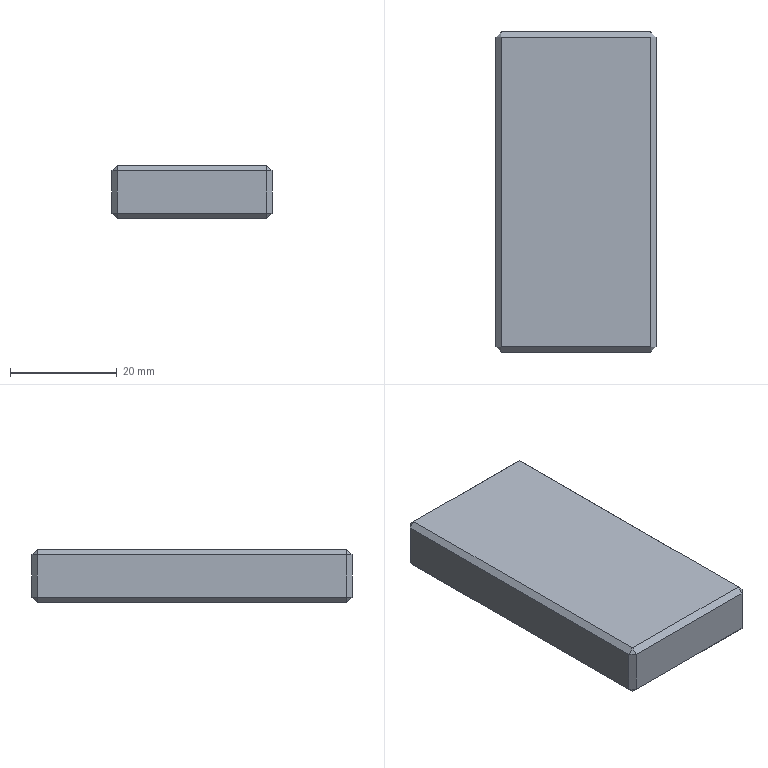Part | STEP file | Planar support spacer block | 1 solid | 26 faces | box 30 x 60 x 10 mm | volume 17805 mm3 | plane 26
STEP:
#1=CARTESIAN_POINT('',(0.,0.,0.));
#2=DIRECTION('',(0.,0.,1.));
#3=DIRECTION('',(1.,0.,0.));
#4=AXIS2_PLACEMENT_3D('',#1,#2,#3);
#5=CARTESIAN_POINT('',(15.,29.,9.));
#6=VERTEX_POINT('',#5);
#7=CARTESIAN_POINT('',(15.,-29.,9.));
#8=VERTEX_POINT('',#7);
#9=CARTESIAN_POINT('',(15.,-30.,9.));
#10=DIRECTION('',(0.,-1.,0.));
#11=VECTOR('',#10,1.);
#12=LINE('',#9,#11);
#13=CARTESIAN_POINT('',(15.,30.,10.));
#14=DIRECTION('',(-1.,0.,0.));
#15=DIRECTION('',(0.,-1.,0.));
#16=AXIS2_PLACEMENT_3D('',#13,#14,#15);
#17=PLANE('',#16);
#18=CARTESIAN_POINT('',(60.,-1.));
#19=DIRECTION('',(1.,0.));
#20=VECTOR('',#19,1.);
#21=LINE('',#18,#20);
#22=(GEOMETRIC_REPRESENTATION_CONTEXT(2)PARAMETRIC_REPRESENTATION_CONTEXT()REPRESENTATION_CONTEXT('',''));
#23=DEFINITIONAL_REPRESENTATION('',(#21),#22);
#24=PCURVE('',#17,#23);
#25=CARTESIAN_POINT('',(14.,0.,10.));
#26=DIRECTION('',(0.7071,0.,0.7071));
#27=DIRECTION('',(0.,-1.,0.));
#28=AXIS2_PLACEMENT_3D('',#25,#26,#27);
#29=PLANE('',#28);
#30=CARTESIAN_POINT('',(30.,1.414));
#31=DIRECTION('',(1.,0.));
#32=VECTOR('',#31,1.);
#33=LINE('',#30,#32);
#34=(GEOMETRIC_REPRESENTATION_CONTEXT(2)PARAMETRIC_REPRESENTATION_CONTEXT()REPRESENTATION_CONTEXT('',''));
#35=DEFINITIONAL_REPRESENTATION('',(#33),#34);
#36=PCURVE('',#29,#35);
#37=SURFACE_CURVE('',#12,(#24,#36),.PCURVE_S1.);
#38=EDGE_CURVE('',#6,#8,#37,.T.);
#39=ORIENTED_EDGE('',*,*,#38,.T.);
#40=CARTESIAN_POINT('',(15.,-29.,1.));
#41=VERTEX_POINT('',#40);
#42=CARTESIAN_POINT('',(15.,-29.,10.));
#43=DIRECTION('',(0.,0.,-1.));
#44=VECTOR('',#43,1.);
#45=LINE('',#42,#44);
#46=CARTESIAN_POINT('',(59.,0.));
#47=DIRECTION('',(0.,-1.));
#48=VECTOR('',#47,1.);
#49=LINE('',#46,#48);
#50=(GEOMETRIC_REPRESENTATION_CONTEXT(2)PARAMETRIC_REPRESENTATION_CONTEXT()REPRESENTATION_CONTEXT('',''));
#51=DEFINITIONAL_REPRESENTATION('',(#49),#50);
#52=PCURVE('',#17,#51);
#53=CARTESIAN_POINT('',(15.,-29.,10.));
#54=DIRECTION('',(-0.7071,0.7071,0.));
#55=DIRECTION('',(0.,0.,-1.));
#56=AXIS2_PLACEMENT_3D('',#53,#54,#55);
#57=PLANE('',#56);
#58=CARTESIAN_POINT('',(0.,0.));
#59=DIRECTION('',(1.,0.));
#60=VECTOR('',#59,1.);
#61=LINE('',#58,#60);
#62=(GEOMETRIC_REPRESENTATION_CONTEXT(2)PARAMETRIC_REPRESENTATION_CONTEXT()REPRESENTATION_CONTEXT('',''));
#63=DEFINITIONAL_REPRESENTATION('',(#61),#62);
#64=PCURVE('',#57,#63);
#65=SURFACE_CURVE('',#45,(#52,#64),.PCURVE_S1.);
#66=EDGE_CURVE('',#8,#41,#65,.T.);
#67=ORIENTED_EDGE('',*,*,#66,.T.);
#68=CARTESIAN_POINT('',(15.,29.,1.));
#69=VERTEX_POINT('',#68);
#70=CARTESIAN_POINT('',(15.,30.,1.));
#71=DIRECTION('',(0.,1.,0.));
#72=VECTOR('',#71,1.);
#73=LINE('',#70,#72);
#74=CARTESIAN_POINT('',(0.,-9.));
#75=DIRECTION('',(-1.,0.));
#76=VECTOR('',#75,1.);
#77=LINE('',#74,#76);
#78=(GEOMETRIC_REPRESENTATION_CONTEXT(2)PARAMETRIC_REPRESENTATION_CONTEXT()REPRESENTATION_CONTEXT('',''));
#79=DEFINITIONAL_REPRESENTATION('',(#77),#78);
#80=PCURVE('',#17,#79);
#81=CARTESIAN_POINT('',(15.,30.,1.));
#82=DIRECTION('',(-0.7071,0.,0.7071));
#83=DIRECTION('',(0.,1.,0.));
#84=AXIS2_PLACEMENT_3D('',#81,#82,#83);
#85=PLANE('',#84);
#86=CARTESIAN_POINT('',(0.,0.));
#87=DIRECTION('',(1.,0.));
#88=VECTOR('',#87,1.);
#89=LINE('',#86,#88);
#90=(GEOMETRIC_REPRESENTATION_CONTEXT(2)PARAMETRIC_REPRESENTATION_CONTEXT()REPRESENTATION_CONTEXT('',''));
#91=DEFINITIONAL_REPRESENTATION('',(#89),#90);
#92=PCURVE('',#85,#91);
#93=SURFACE_CURVE('',#73,(#80,#92),.PCURVE_S1.);
#94=EDGE_CURVE('',#41,#69,#93,.T.);
#95=ORIENTED_EDGE('',*,*,#94,.T.);
#96=CARTESIAN_POINT('',(15.,29.,10.));
#97=DIRECTION('',(0.,0.,1.));
#98=VECTOR('',#97,1.);
#99=LINE('',#96,#98);
#100=CARTESIAN_POINT('',(1.,0.));
#101=DIRECTION('',(0.,1.));
#102=VECTOR('',#101,1.);
#103=LINE('',#100,#102);
#104=(GEOMETRIC_REPRESENTATION_CONTEXT(2)PARAMETRIC_REPRESENTATION_CONTEXT()REPRESENTATION_CONTEXT('',''));
#105=DEFINITIONAL_REPRESENTATION('',(#103),#104);
#106=PCURVE('',#17,#105);
#107=CARTESIAN_POINT('',(14.,30.,10.));
#108=DIRECTION('',(-0.7071,-0.7071,0.));
#109=DIRECTION('',(0.,0.,-1.));
#110=AXIS2_PLACEMENT_3D('',#107,#108,#109);
#111=PLANE('',#110);
#112=CARTESIAN_POINT('',(0.,1.414));
#113=DIRECTION('',(-1.,0.));
#114=VECTOR('',#113,1.);
#115=LINE('',#112,#114);
#116=(GEOMETRIC_REPRESENTATION_CONTEXT(2)PARAMETRIC_REPRESENTATION_CONTEXT()REPRESENTATION_CONTEXT('',''));
#117=DEFINITIONAL_REPRESENTATION('',(#115),#116);
#118=PCURVE('',#111,#117);
#119=SURFACE_CURVE('',#99,(#106,#118),.PCURVE_S1.);
#120=EDGE_CURVE('',#69,#6,#119,.T.);
#121=ORIENTED_EDGE('',*,*,#120,.T.);
#122=EDGE_LOOP('',(#39,#67,#95,#121));
#123=FACE_BOUND('',#122,.T.);
#124=ADVANCED_FACE('',(#123),#17,.F.);
#125=CARTESIAN_POINT('',(14.,30.,9.));
#126=VERTEX_POINT('',#125);
#127=CARTESIAN_POINT('',(14.,30.,1.));
#128=VERTEX_POINT('',#127);
#129=CARTESIAN_POINT('',(14.,30.,10.));
#130=DIRECTION('',(0.,0.,-1.));
#131=VECTOR('',#130,1.);
#132=LINE('',#129,#131);
#133=CARTESIAN_POINT('',(-15.,30.,10.));
#134=DIRECTION('',(0.,-1.,0.));
#135=DIRECTION('',(0.,0.,-1.));
#136=AXIS2_PLACEMENT_3D('',#133,#134,#135);
#137=PLANE('',#136);
#138=CARTESIAN_POINT('',(0.,29.));
#139=DIRECTION('',(1.,0.));
#140=VECTOR('',#139,1.);
#141=LINE('',#138,#140);
#142=(GEOMETRIC_REPRESENTATION_CONTEXT(2)PARAMETRIC_REPRESENTATION_CONTEXT()REPRESENTATION_CONTEXT('',''));
#143=DEFINITIONAL_REPRESENTATION('',(#141),#142);
#144=PCURVE('',#137,#143);
#145=CARTESIAN_POINT('',(0.,0.));
#146=DIRECTION('',(1.,0.));
#147=VECTOR('',#146,1.);
#148=LINE('',#145,#147);
#149=(GEOMETRIC_REPRESENTATION_CONTEXT(2)PARAMETRIC_REPRESENTATION_CONTEXT()REPRESENTATION_CONTEXT('',''));
#150=DEFINITIONAL_REPRESENTATION('',(#148),#149);
#151=PCURVE('',#111,#150);
#152=SURFACE_CURVE('',#132,(#144,#151),.PCURVE_S1.);
#153=EDGE_CURVE('',#126,#128,#152,.T.);
#154=ORIENTED_EDGE('',*,*,#153,.T.);
#155=CARTESIAN_POINT('',(-14.,30.,1.));
#156=VERTEX_POINT('',#155);
#157=CARTESIAN_POINT('',(-15.,30.,1.));
#158=DIRECTION('',(-1.,0.,0.));
#159=VECTOR('',#158,1.);
#160=LINE('',#157,#159);
#161=CARTESIAN_POINT('',(9.,0.));
#162=DIRECTION('',(0.,-1.));
#163=VECTOR('',#162,1.);
#164=LINE('',#161,#163);
#165=(GEOMETRIC_REPRESENTATION_CONTEXT(2)PARAMETRIC_REPRESENTATION_CONTEXT()REPRESENTATION_CONTEXT('',''));
#166=DEFINITIONAL_REPRESENTATION('',(#164),#165);
#167=PCURVE('',#137,#166);
#168=CARTESIAN_POINT('',(-15.,30.,1.));
#169=DIRECTION('',(0.,-0.7071,0.7071));
#170=DIRECTION('',(-1.,0.,0.));
#171=AXIS2_PLACEMENT_3D('',#168,#169,#170);
#172=PLANE('',#171);
#173=CARTESIAN_POINT('',(0.,0.));
#174=DIRECTION('',(1.,0.));
#175=VECTOR('',#174,1.);
#176=LINE('',#173,#175);
#177=(GEOMETRIC_REPRESENTATION_CONTEXT(2)PARAMETRIC_REPRESENTATION_CONTEXT()REPRESENTATION_CONTEXT('',''));
#178=DEFINITIONAL_REPRESENTATION('',(#176),#177);
#179=PCURVE('',#172,#178);
#180=SURFACE_CURVE('',#160,(#167,#179),.PCURVE_S1.);
#181=EDGE_CURVE('',#128,#156,#180,.T.);
#182=ORIENTED_EDGE('',*,*,#181,.T.);
#183=CARTESIAN_POINT('',(-14.,30.,9.));
#184=VERTEX_POINT('',#183);
#185=CARTESIAN_POINT('',(-14.,30.,10.));
#186=DIRECTION('',(0.,0.,1.));
#187=VECTOR('',#186,1.);
#188=LINE('',#185,#187);
#189=CARTESIAN_POINT('',(0.,1.));
#190=DIRECTION('',(-1.,0.));
#191=VECTOR('',#190,1.);
#192=LINE('',#189,#191);
#193=(GEOMETRIC_REPRESENTATION_CONTEXT(2)PARAMETRIC_REPRESENTATION_CONTEXT()REPRESENTATION_CONTEXT('',''));
#194=DEFINITIONAL_REPRESENTATION('',(#192),#193);
#195=PCURVE('',#137,#194);
#196=CARTESIAN_POINT('',(-15.,29.,10.));
#197=DIRECTION('',(0.7071,-0.7071,0.));
#198=DIRECTION('',(0.,0.,-1.));
#199=AXIS2_PLACEMENT_3D('',#196,#197,#198);
#200=PLANE('',#199);
#201=CARTESIAN_POINT('',(0.,1.414));
#202=DIRECTION('',(-1.,0.));
#203=VECTOR('',#202,1.);
#204=LINE('',#201,#203);
#205=(GEOMETRIC_REPRESENTATION_CONTEXT(2)PARAMETRIC_REPRESENTATION_CONTEXT()REPRESENTATION_CONTEXT('',''));
#206=DEFINITIONAL_REPRESENTATION('',(#204),#205);
#207=PCURVE('',#200,#206);
#208=SURFACE_CURVE('',#188,(#195,#207),.PCURVE_S1.);
#209=EDGE_CURVE('',#156,#184,#208,.T.);
#210=ORIENTED_EDGE('',*,*,#209,.T.);
#211=CARTESIAN_POINT('',(15.,30.,9.));
#212=DIRECTION('',(1.,0.,0.));
#213=VECTOR('',#212,1.);
#214=LINE('',#211,#213);
#215=CARTESIAN_POINT('',(1.,30.));
#216=DIRECTION('',(0.,1.));
#217=VECTOR('',#216,1.);
#218=LINE('',#215,#217);
#219=(GEOMETRIC_REPRESENTATION_CONTEXT(2)PARAMETRIC_REPRESENTATION_CONTEXT()REPRESENTATION_CONTEXT('',''));
#220=DEFINITIONAL_REPRESENTATION('',(#218),#219);
#221=PCURVE('',#137,#220);
#222=CARTESIAN_POINT('',(0.,29.,10.));
#223=DIRECTION('',(0.,0.7071,0.7071));
#224=DIRECTION('',(1.,0.,0.));
#225=AXIS2_PLACEMENT_3D('',#222,#223,#224);
#226=PLANE('',#225);
#227=CARTESIAN_POINT('',(15.,1.414));
#228=DIRECTION('',(1.,0.));
#229=VECTOR('',#228,1.);
#230=LINE('',#227,#229);
#231=(GEOMETRIC_REPRESENTATION_CONTEXT(2)PARAMETRIC_REPRESENTATION_CONTEXT()REPRESENTATION_CONTEXT('',''));
#232=DEFINITIONAL_REPRESENTATION('',(#230),#231);
#233=PCURVE('',#226,#232);
#234=SURFACE_CURVE('',#214,(#221,#233),.PCURVE_S1.);
#235=EDGE_CURVE('',#184,#126,#234,.T.);
#236=ORIENTED_EDGE('',*,*,#235,.T.);
#237=EDGE_LOOP('',(#154,#182,#210,#236));
#238=FACE_BOUND('',#237,.T.);
#239=ADVANCED_FACE('',(#238),#137,.F.);
#240=CARTESIAN_POINT('',(-15.,29.,9.));
#241=VERTEX_POINT('',#240);
#242=CARTESIAN_POINT('',(-15.,29.,1.));
#243=VERTEX_POINT('',#242);
#244=CARTESIAN_POINT('',(-15.,29.,10.));
#245=DIRECTION('',(0.,0.,-1.));
#246=VECTOR('',#245,1.);
#247=LINE('',#244,#246);
#248=CARTESIAN_POINT('',(-15.,30.,10.));
#249=DIRECTION('',(1.,0.,0.));
#250=DIRECTION('',(0.,1.,0.));
#251=AXIS2_PLACEMENT_3D('',#248,#249,#250);
#252=PLANE('',#251);
#253=CARTESIAN_POINT('',(-1.,0.));
#254=DIRECTION('',(0.,-1.));
#255=VECTOR('',#254,1.);
#256=LINE('',#253,#255);
#257=(GEOMETRIC_REPRESENTATION_CONTEXT(2)PARAMETRIC_REPRESENTATION_CONTEXT()REPRESENTATION_CONTEXT('',''));
#258=DEFINITIONAL_REPRESENTATION('',(#256),#257);
#259=PCURVE('',#252,#258);
#260=CARTESIAN_POINT('',(0.,0.));
#261=DIRECTION('',(1.,0.));
#262=VECTOR('',#261,1.);
#263=LINE('',#260,#262);
#264=(GEOMETRIC_REPRESENTATION_CONTEXT(2)PARAMETRIC_REPRESENTATION_CONTEXT()REPRESENTATION_CONTEXT('',''));
#265=DEFINITIONAL_REPRESENTATION('',(#263),#264);
#266=PCURVE('',#200,#265);
#267=SURFACE_CURVE('',#247,(#259,#266),.PCURVE_S1.);
#268=EDGE_CURVE('',#241,#243,#267,.T.);
#269=ORIENTED_EDGE('',*,*,#268,.T.);
#270=CARTESIAN_POINT('',(-15.,-29.,1.));
#271=VERTEX_POINT('',#270);
#272=CARTESIAN_POINT('',(-15.,30.,1.));
#273=DIRECTION('',(0.,-1.,0.));
#274=VECTOR('',#273,1.);
#275=LINE('',#272,#274);
#276=CARTESIAN_POINT('',(0.,-9.));
#277=DIRECTION('',(-1.,0.));
#278=VECTOR('',#277,1.);
#279=LINE('',#276,#278);
#280=(GEOMETRIC_REPRESENTATION_CONTEXT(2)PARAMETRIC_REPRESENTATION_CONTEXT()REPRESENTATION_CONTEXT('',''));
#281=DEFINITIONAL_REPRESENTATION('',(#279),#280);
#282=PCURVE('',#252,#281);
#283=CARTESIAN_POINT('',(-15.,30.,1.));
#284=DIRECTION('',(0.7071,0.,0.7071));
#285=DIRECTION('',(0.,-1.,0.));
#286=AXIS2_PLACEMENT_3D('',#283,#284,#285);
#287=PLANE('',#286);
#288=CARTESIAN_POINT('',(0.,0.));
#289=DIRECTION('',(1.,0.));
#290=VECTOR('',#289,1.);
#291=LINE('',#288,#290);
#292=(GEOMETRIC_REPRESENTATION_CONTEXT(2)PARAMETRIC_REPRESENTATION_CONTEXT()REPRESENTATION_CONTEXT('',''));
#293=DEFINITIONAL_REPRESENTATION('',(#291),#292);
#294=PCURVE('',#287,#293);
#295=SURFACE_CURVE('',#275,(#282,#294),.PCURVE_S1.);
#296=EDGE_CURVE('',#243,#271,#295,.T.);
#297=ORIENTED_EDGE('',*,*,#296,.T.);
#298=CARTESIAN_POINT('',(-15.,-29.,9.));
#299=VERTEX_POINT('',#298);
#300=CARTESIAN_POINT('',(-15.,-29.,10.));
#301=DIRECTION('',(0.,0.,1.));
#302=VECTOR('',#301,1.);
#303=LINE('',#300,#302);
#304=CARTESIAN_POINT('',(-59.,0.));
#305=DIRECTION('',(0.,1.));
#306=VECTOR('',#305,1.);
#307=LINE('',#304,#306);
#308=(GEOMETRIC_REPRESENTATION_CONTEXT(2)PARAMETRIC_REPRESENTATION_CONTEXT()REPRESENTATION_CONTEXT('',''));
#309=DEFINITIONAL_REPRESENTATION('',(#307),#308);
#310=PCURVE('',#252,#309);
#311=CARTESIAN_POINT('',(-14.,-30.,10.));
#312=DIRECTION('',(0.7071,0.7071,0.));
#313=DIRECTION('',(0.,0.,-1.));
#314=AXIS2_PLACEMENT_3D('',#311,#312,#313);
#315=PLANE('',#314);
#316=CARTESIAN_POINT('',(0.,1.414));
#317=DIRECTION('',(-1.,0.));
#318=VECTOR('',#317,1.);
#319=LINE('',#316,#318);
#320=(GEOMETRIC_REPRESENTATION_CONTEXT(2)PARAMETRIC_REPRESENTATION_CONTEXT()REPRESENTATION_CONTEXT('',''));
#321=DEFINITIONAL_REPRESENTATION('',(#319),#320);
#322=PCURVE('',#315,#321);
#323=SURFACE_CURVE('',#303,(#310,#322),.PCURVE_S1.);
#324=EDGE_CURVE('',#271,#299,#323,.T.);
#325=ORIENTED_EDGE('',*,*,#324,.T.);
#326=CARTESIAN_POINT('',(-15.,30.,9.));
#327=DIRECTION('',(0.,1.,0.));
#328=VECTOR('',#327,1.);
#329=LINE('',#326,#328);
#330=CARTESIAN_POINT('',(0.,-1.));
#331=DIRECTION('',(1.,0.));
#332=VECTOR('',#331,1.);
#333=LINE('',#330,#332);
#334=(GEOMETRIC_REPRESENTATION_CONTEXT(2)PARAMETRIC_REPRESENTATION_CONTEXT()REPRESENTATION_CONTEXT('',''));
#335=DEFINITIONAL_REPRESENTATION('',(#333),#334);
#336=PCURVE('',#252,#335);
#337=CARTESIAN_POINT('',(-14.,0.,10.));
#338=DIRECTION('',(-0.7071,0.,0.7071));
#339=DIRECTION('',(0.,1.,0.));
#340=AXIS2_PLACEMENT_3D('',#337,#338,#339);
#341=PLANE('',#340);
#342=CARTESIAN_POINT('',(30.,1.414));
#343=DIRECTION('',(1.,0.));
#344=VECTOR('',#343,1.);
#345=LINE('',#342,#344);
#346=(GEOMETRIC_REPRESENTATION_CONTEXT(2)PARAMETRIC_REPRESENTATION_CONTEXT()REPRESENTATION_CONTEXT('',''));
#347=DEFINITIONAL_REPRESENTATION('',(#345),#346);
#348=PCURVE('',#341,#347);
#349=SURFACE_CURVE('',#329,(#336,#348),.PCURVE_S1.);
#350=EDGE_CURVE('',#299,#241,#349,.T.);
#351=ORIENTED_EDGE('',*,*,#350,.T.);
#352=EDGE_LOOP('',(#269,#297,#325,#351));
#353=FACE_BOUND('',#352,.T.);
#354=ADVANCED_FACE('',(#353),#252,.F.);
#355=CARTESIAN_POINT('',(-14.,-30.,9.));
#356=VERTEX_POINT('',#355);
#357=CARTESIAN_POINT('',(-14.,-30.,1.));
#358=VERTEX_POINT('',#357);
#359=CARTESIAN_POINT('',(-14.,-30.,10.));
#360=DIRECTION('',(0.,0.,-1.));
#361=VECTOR('',#360,1.);
#362=LINE('',#359,#361);
#363=CARTESIAN_POINT('',(-15.,-30.,10.));
#364=DIRECTION('',(0.,1.,0.));
#365=DIRECTION('',(0.,0.,1.));
#366=AXIS2_PLACEMENT_3D('',#363,#364,#365);
#367=PLANE('',#366);
#368=CARTESIAN_POINT('',(0.,1.));
#369=DIRECTION('',(-1.,0.));
#370=VECTOR('',#369,1.);
#371=LINE('',#368,#370);
#372=(GEOMETRIC_REPRESENTATION_CONTEXT(2)PARAMETRIC_REPRESENTATION_CONTEXT()REPRESENTATION_CONTEXT('',''));
#373=DEFINITIONAL_REPRESENTATION('',(#371),#372);
#374=PCURVE('',#367,#373);
#375=CARTESIAN_POINT('',(0.,0.));
#376=DIRECTION('',(1.,0.));
#377=VECTOR('',#376,1.);
#378=LINE('',#375,#377);
#379=(GEOMETRIC_REPRESENTATION_CONTEXT(2)PARAMETRIC_REPRESENTATION_CONTEXT()REPRESENTATION_CONTEXT('',''));
#380=DEFINITIONAL_REPRESENTATION('',(#378),#379);
#381=PCURVE('',#315,#380);
#382=SURFACE_CURVE('',#362,(#374,#381),.PCURVE_S1.);
#383=EDGE_CURVE('',#356,#358,#382,.T.);
#384=ORIENTED_EDGE('',*,*,#383,.T.);
#385=CARTESIAN_POINT('',(14.,-30.,1.));
#386=VERTEX_POINT('',#385);
#387=CARTESIAN_POINT('',(-15.,-30.,1.));
#388=DIRECTION('',(1.,0.,0.));
#389=VECTOR('',#388,1.);
#390=LINE('',#387,#389);
#391=CARTESIAN_POINT('',(-9.,0.));
#392=DIRECTION('',(0.,1.));
#393=VECTOR('',#392,1.);
#394=LINE('',#391,#393);
#395=(GEOMETRIC_REPRESENTATION_CONTEXT(2)PARAMETRIC_REPRESENTATION_CONTEXT()REPRESENTATION_CONTEXT('',''));
#396=DEFINITIONAL_REPRESENTATION('',(#394),#395);
#397=PCURVE('',#367,#396);
#398=CARTESIAN_POINT('',(-15.,-30.,1.));
#399=DIRECTION('',(0.,0.7071,0.7071));
#400=DIRECTION('',(1.,0.,0.));
#401=AXIS2_PLACEMENT_3D('',#398,#399,#400);
#402=PLANE('',#401);
#403=CARTESIAN_POINT('',(0.,0.));
#404=DIRECTION('',(1.,0.));
#405=VECTOR('',#404,1.);
#406=LINE('',#403,#405);
#407=(GEOMETRIC_REPRESENTATION_CONTEXT(2)PARAMETRIC_REPRESENTATION_CONTEXT()REPRESENTATION_CONTEXT('',''));
#408=DEFINITIONAL_REPRESENTATION('',(#406),#407);
#409=PCURVE('',#402,#408);
#410=SURFACE_CURVE('',#390,(#397,#409),.PCURVE_S1.);
#411=EDGE_CURVE('',#358,#386,#410,.T.);
#412=ORIENTED_EDGE('',*,*,#411,.T.);
#413=CARTESIAN_POINT('',(14.,-30.,9.));
#414=VERTEX_POINT('',#413);
#415=CARTESIAN_POINT('',(14.,-30.,10.));
#416=DIRECTION('',(0.,0.,1.));
#417=VECTOR('',#416,1.);
#418=LINE('',#415,#417);
#419=CARTESIAN_POINT('',(0.,29.));
#420=DIRECTION('',(1.,0.));
#421=VECTOR('',#420,1.);
#422=LINE('',#419,#421);
#423=(GEOMETRIC_REPRESENTATION_CONTEXT(2)PARAMETRIC_REPRESENTATION_CONTEXT()REPRESENTATION_CONTEXT('',''));
#424=DEFINITIONAL_REPRESENTATION('',(#422),#423);
#425=PCURVE('',#367,#424);
#426=CARTESIAN_POINT('',(0.,1.414));
#427=DIRECTION('',(-1.,0.));
#428=VECTOR('',#427,1.);
#429=LINE('',#426,#428);
#430=(GEOMETRIC_REPRESENTATION_CONTEXT(2)PARAMETRIC_REPRESENTATION_CONTEXT()REPRESENTATION_CONTEXT('',''));
#431=DEFINITIONAL_REPRESENTATION('',(#429),#430);
#432=PCURVE('',#57,#431);
#433=SURFACE_CURVE('',#418,(#425,#432),.PCURVE_S1.);
#434=EDGE_CURVE('',#386,#414,#433,.T.);
#435=ORIENTED_EDGE('',*,*,#434,.T.);
#436=CARTESIAN_POINT('',(-15.,-30.,9.));
#437=DIRECTION('',(-1.,0.,0.));
#438=VECTOR('',#437,1.);
#439=LINE('',#436,#438);
#440=CARTESIAN_POINT('',(-1.,0.));
#441=DIRECTION('',(0.,-1.));
#442=VECTOR('',#441,1.);
#443=LINE('',#440,#442);
#444=(GEOMETRIC_REPRESENTATION_CONTEXT(2)PARAMETRIC_REPRESENTATION_CONTEXT()REPRESENTATION_CONTEXT('',''));
#445=DEFINITIONAL_REPRESENTATION('',(#443),#444);
#446=PCURVE('',#367,#445);
#447=CARTESIAN_POINT('',(0.,-29.,10.));
#448=DIRECTION('',(0.,-0.7071,0.7071));
#449=DIRECTION('',(-1.,0.,0.));
#450=AXIS2_PLACEMENT_3D('',#447,#448,#449);
#451=PLANE('',#450);
#452=CARTESIAN_POINT('',(15.,1.414));
#453=DIRECTION('',(1.,0.));
#454=VECTOR('',#453,1.);
#455=LINE('',#452,#454);
#456=(GEOMETRIC_REPRESENTATION_CONTEXT(2)PARAMETRIC_REPRESENTATION_CONTEXT()REPRESENTATION_CONTEXT('',''));
#457=DEFINITIONAL_REPRESENTATION('',(#455),#456);
#458=PCURVE('',#451,#457);
#459=SURFACE_CURVE('',#439,(#446,#458),.PCURVE_S1.);
#460=EDGE_CURVE('',#414,#356,#459,.T.);
#461=ORIENTED_EDGE('',*,*,#460,.T.);
#462=EDGE_LOOP('',(#384,#412,#435,#461));
#463=FACE_BOUND('',#462,.T.);
#464=ADVANCED_FACE('',(#463),#367,.F.);
#465=CARTESIAN_POINT('',(-14.,-29.,10.));
#466=VERTEX_POINT('',#465);
#467=CARTESIAN_POINT('',(14.,-29.,10.));
#468=VERTEX_POINT('',#467);
#469=CARTESIAN_POINT('',(15.,-29.,10.));
#470=DIRECTION('',(1.,0.,0.));
#471=VECTOR('',#470,1.);
#472=LINE('',#469,#471);
#473=CARTESIAN_POINT('',(0.,0.,10.));
#474=DIRECTION('',(0.,0.,1.));
#475=DIRECTION('',(1.,0.,0.));
#476=AXIS2_PLACEMENT_3D('',#473,#474,#475);
#477=PLANE('',#476);
#478=CARTESIAN_POINT('',(15.,-29.));
#479=DIRECTION('',(1.,0.));
#480=VECTOR('',#479,1.);
#481=LINE('',#478,#480);
#482=(GEOMETRIC_REPRESENTATION_CONTEXT(2)PARAMETRIC_REPRESENTATION_CONTEXT()REPRESENTATION_CONTEXT('',''));
#483=DEFINITIONAL_REPRESENTATION('',(#481),#482);
#484=PCURVE('',#477,#483);
#485=CARTESIAN_POINT('',(-15.,0.));
#486=DIRECTION('',(-1.,0.));
#487=VECTOR('',#486,1.);
#488=LINE('',#485,#487);
#489=(GEOMETRIC_REPRESENTATION_CONTEXT(2)PARAMETRIC_REPRESENTATION_CONTEXT()REPRESENTATION_CONTEXT('',''));
#490=DEFINITIONAL_REPRESENTATION('',(#488),#489);
#491=PCURVE('',#451,#490);
#492=SURFACE_CURVE('',#472,(#484,#491),.PCURVE_S1.);
#493=EDGE_CURVE('',#466,#468,#492,.T.);
#494=ORIENTED_EDGE('',*,*,#493,.T.);
#495=CARTESIAN_POINT('',(14.,29.,10.));
#496=VERTEX_POINT('',#495);
#497=CARTESIAN_POINT('',(14.,30.,10.));
#498=DIRECTION('',(0.,1.,0.));
#499=VECTOR('',#498,1.);
#500=LINE('',#497,#499);
#501=CARTESIAN_POINT('',(14.,30.));
#502=DIRECTION('',(0.,1.));
#503=VECTOR('',#502,1.);
#504=LINE('',#501,#503);
#505=(GEOMETRIC_REPRESENTATION_CONTEXT(2)PARAMETRIC_REPRESENTATION_CONTEXT()REPRESENTATION_CONTEXT('',''));
#506=DEFINITIONAL_REPRESENTATION('',(#504),#505);
#507=PCURVE('',#477,#506);
#508=CARTESIAN_POINT('',(-30.,0.));
#509=DIRECTION('',(-1.,0.));
#510=VECTOR('',#509,1.);
#511=LINE('',#508,#510);
#512=(GEOMETRIC_REPRESENTATION_CONTEXT(2)PARAMETRIC_REPRESENTATION_CONTEXT()REPRESENTATION_CONTEXT('',''));
#513=DEFINITIONAL_REPRESENTATION('',(#511),#512);
#514=PCURVE('',#29,#513);
#515=SURFACE_CURVE('',#500,(#507,#514),.PCURVE_S1.);
#516=EDGE_CURVE('',#468,#496,#515,.T.);
#517=ORIENTED_EDGE('',*,*,#516,.T.);
#518=CARTESIAN_POINT('',(-14.,29.,10.));
#519=VERTEX_POINT('',#518);
#520=CARTESIAN_POINT('',(-15.,29.,10.));
#521=DIRECTION('',(-1.,0.,0.));
#522=VECTOR('',#521,1.);
#523=LINE('',#520,#522);
#524=CARTESIAN_POINT('',(-15.,29.));
#525=DIRECTION('',(-1.,0.));
#526=VECTOR('',#525,1.);
#527=LINE('',#524,#526);
#528=(GEOMETRIC_REPRESENTATION_CONTEXT(2)PARAMETRIC_REPRESENTATION_CONTEXT()REPRESENTATION_CONTEXT('',''));
#529=DEFINITIONAL_REPRESENTATION('',(#527),#528);
#530=PCURVE('',#477,#529);
#531=CARTESIAN_POINT('',(-15.,0.));
#532=DIRECTION('',(-1.,0.));
#533=VECTOR('',#532,1.);
#534=LINE('',#531,#533);
#535=(GEOMETRIC_REPRESENTATION_CONTEXT(2)PARAMETRIC_REPRESENTATION_CONTEXT()REPRESENTATION_CONTEXT('',''));
#536=DEFINITIONAL_REPRESENTATION('',(#534),#535);
#537=PCURVE('',#226,#536);
#538=SURFACE_CURVE('',#523,(#530,#537),.PCURVE_S1.);
#539=EDGE_CURVE('',#496,#519,#538,.T.);
#540=ORIENTED_EDGE('',*,*,#539,.T.);
#541=CARTESIAN_POINT('',(-14.,-30.,10.));
#542=DIRECTION('',(0.,-1.,0.));
#543=VECTOR('',#542,1.);
#544=LINE('',#541,#543);
#545=CARTESIAN_POINT('',(-14.,-30.));
#546=DIRECTION('',(0.,-1.));
#547=VECTOR('',#546,1.);
#548=LINE('',#545,#547);
#549=(GEOMETRIC_REPRESENTATION_CONTEXT(2)PARAMETRIC_REPRESENTATION_CONTEXT()REPRESENTATION_CONTEXT('',''));
#550=DEFINITIONAL_REPRESENTATION('',(#548),#549);
#551=PCURVE('',#477,#550);
#552=CARTESIAN_POINT('',(-30.,0.));
#553=DIRECTION('',(-1.,0.));
#554=VECTOR('',#553,1.);
#555=LINE('',#552,#554);
#556=(GEOMETRIC_REPRESENTATION_CONTEXT(2)PARAMETRIC_REPRESENTATION_CONTEXT()REPRESENTATION_CONTEXT('',''));
#557=DEFINITIONAL_REPRESENTATION('',(#555),#556);
#558=PCURVE('',#341,#557);
#559=SURFACE_CURVE('',#544,(#551,#558),.PCURVE_S1.);
#560=EDGE_CURVE('',#519,#466,#559,.T.);
#561=ORIENTED_EDGE('',*,*,#560,.T.);
#562=EDGE_LOOP('',(#494,#517,#540,#561));
#563=FACE_BOUND('',#562,.T.);
#564=ADVANCED_FACE('',(#563),#477,.T.);
#565=CARTESIAN_POINT('',(-14.,29.,0.));
#566=VERTEX_POINT('',#565);
#567=CARTESIAN_POINT('',(14.,29.,0.));
#568=VERTEX_POINT('',#567);
#569=CARTESIAN_POINT('',(0.,29.,0.));
#570=DIRECTION('',(1.,0.,0.));
#571=VECTOR('',#570,1.);
#572=LINE('',#569,#571);
#573=CARTESIAN_POINT('',(0.,0.,0.));
#574=DIRECTION('',(0.,0.,1.));
#575=DIRECTION('',(1.,0.,0.));
#576=AXIS2_PLACEMENT_3D('',#573,#574,#575);
#577=PLANE('',#576);
#578=CARTESIAN_POINT('',(0.,29.));
#579=DIRECTION('',(1.,0.));
#580=VECTOR('',#579,1.);
#581=LINE('',#578,#580);
#582=(GEOMETRIC_REPRESENTATION_CONTEXT(2)PARAMETRIC_REPRESENTATION_CONTEXT()REPRESENTATION_CONTEXT('',''));
#583=DEFINITIONAL_REPRESENTATION('',(#581),#582);
#584=PCURVE('',#577,#583);
#585=CARTESIAN_POINT('',(-15.,1.414));
#586=DIRECTION('',(-1.,0.));
#587=VECTOR('',#586,1.);
#588=LINE('',#585,#587);
#589=(GEOMETRIC_REPRESENTATION_CONTEXT(2)PARAMETRIC_REPRESENTATION_CONTEXT()REPRESENTATION_CONTEXT('',''));
#590=DEFINITIONAL_REPRESENTATION('',(#588),#589);
#591=PCURVE('',#172,#590);
#592=SURFACE_CURVE('',#572,(#584,#591),.PCURVE_S1.);
#593=EDGE_CURVE('',#566,#568,#592,.T.);
#594=ORIENTED_EDGE('',*,*,#593,.T.);
#595=CARTESIAN_POINT('',(14.,-29.,0.));
#596=VERTEX_POINT('',#595);
#597=CARTESIAN_POINT('',(14.,0.,0.));
#598=DIRECTION('',(0.,-1.,0.));
#599=VECTOR('',#598,1.);
#600=LINE('',#597,#599);
#601=CARTESIAN_POINT('',(14.,0.));
#602=DIRECTION('',(0.,-1.));
#603=VECTOR('',#602,1.);
#604=LINE('',#601,#603);
#605=(GEOMETRIC_REPRESENTATION_CONTEXT(2)PARAMETRIC_REPRESENTATION_CONTEXT()REPRESENTATION_CONTEXT('',''));
#606=DEFINITIONAL_REPRESENTATION('',(#604),#605);
#607=PCURVE('',#577,#606);
#608=CARTESIAN_POINT('',(-30.,1.414));
#609=DIRECTION('',(-1.,0.));
#610=VECTOR('',#609,1.);
#611=LINE('',#608,#610);
#612=(GEOMETRIC_REPRESENTATION_CONTEXT(2)PARAMETRIC_REPRESENTATION_CONTEXT()REPRESENTATION_CONTEXT('',''));
#613=DEFINITIONAL_REPRESENTATION('',(#611),#612);
#614=PCURVE('',#85,#613);
#615=SURFACE_CURVE('',#600,(#607,#614),.PCURVE_S1.);
#616=EDGE_CURVE('',#568,#596,#615,.T.);
#617=ORIENTED_EDGE('',*,*,#616,.T.);
#618=CARTESIAN_POINT('',(-14.,-29.,0.));
#619=VERTEX_POINT('',#618);
#620=CARTESIAN_POINT('',(0.,-29.,0.));
#621=DIRECTION('',(-1.,0.,0.));
#622=VECTOR('',#621,1.);
#623=LINE('',#620,#622);
#624=CARTESIAN_POINT('',(0.,-29.));
#625=DIRECTION('',(-1.,0.));
#626=VECTOR('',#625,1.);
#627=LINE('',#624,#626);
#628=(GEOMETRIC_REPRESENTATION_CONTEXT(2)PARAMETRIC_REPRESENTATION_CONTEXT()REPRESENTATION_CONTEXT('',''));
#629=DEFINITIONAL_REPRESENTATION('',(#627),#628);
#630=PCURVE('',#577,#629);
#631=CARTESIAN_POINT('',(15.,1.414));
#632=DIRECTION('',(-1.,0.));
#633=VECTOR('',#632,1.);
#634=LINE('',#631,#633);
#635=(GEOMETRIC_REPRESENTATION_CONTEXT(2)PARAMETRIC_REPRESENTATION_CONTEXT()REPRESENTATION_CONTEXT('',''));
#636=DEFINITIONAL_REPRESENTATION('',(#634),#635);
#637=PCURVE('',#402,#636);
#638=SURFACE_CURVE('',#623,(#630,#637),.PCURVE_S1.);
#639=EDGE_CURVE('',#596,#619,#638,.T.);
#640=ORIENTED_EDGE('',*,*,#639,.T.);
#641=CARTESIAN_POINT('',(-14.,0.,0.));
#642=DIRECTION('',(0.,1.,0.));
#643=VECTOR('',#642,1.);
#644=LINE('',#641,#643);
#645=CARTESIAN_POINT('',(-14.,0.));
#646=DIRECTION('',(0.,1.));
#647=VECTOR('',#646,1.);
#648=LINE('',#645,#647);
#649=(GEOMETRIC_REPRESENTATION_CONTEXT(2)PARAMETRIC_REPRESENTATION_CONTEXT()REPRESENTATION_CONTEXT('',''));
#650=DEFINITIONAL_REPRESENTATION('',(#648),#649);
#651=PCURVE('',#577,#650);
#652=CARTESIAN_POINT('',(30.,1.414));
#653=DIRECTION('',(-1.,0.));
#654=VECTOR('',#653,1.);
#655=LINE('',#652,#654);
#656=(GEOMETRIC_REPRESENTATION_CONTEXT(2)PARAMETRIC_REPRESENTATION_CONTEXT()REPRESENTATION_CONTEXT('',''));
#657=DEFINITIONAL_REPRESENTATION('',(#655),#656);
#658=PCURVE('',#287,#657);
#659=SURFACE_CURVE('',#644,(#651,#658),.PCURVE_S1.);
#660=EDGE_CURVE('',#619,#566,#659,.T.);
#661=ORIENTED_EDGE('',*,*,#660,.T.);
#662=EDGE_LOOP('',(#594,#617,#640,#661));
#663=FACE_BOUND('',#662,.T.);
#664=ADVANCED_FACE('',(#663),#577,.F.);
#665=CARTESIAN_POINT('',(-14.5,-29.,9.5));
#666=DIRECTION('',(-0.7071,0.,-0.7071));
#667=VECTOR('',#666,1.);
#668=LINE('',#665,#667);
#669=CARTESIAN_POINT('',(-29.,0.7071));
#670=DIRECTION('',(0.,1.));
#671=VECTOR('',#670,1.);
#672=LINE('',#669,#671);
#673=(GEOMETRIC_REPRESENTATION_CONTEXT(2)PARAMETRIC_REPRESENTATION_CONTEXT()REPRESENTATION_CONTEXT('',''));
#674=DEFINITIONAL_REPRESENTATION('',(#672),#673);
#675=PCURVE('',#341,#674);
#676=CARTESIAN_POINT('',(-14.,-30.,9.));
#677=DIRECTION('',(-0.5774,-0.5774,0.5774));
#678=DIRECTION('',(0.7071,0.,0.7071));
#679=AXIS2_PLACEMENT_3D('',#676,#677,#678);
#680=PLANE('',#679);
#681=CARTESIAN_POINT('',(0.,1.225));
#682=DIRECTION('',(-1.,0.));
#683=VECTOR('',#682,1.);
#684=LINE('',#681,#683);
#685=(GEOMETRIC_REPRESENTATION_CONTEXT(2)PARAMETRIC_REPRESENTATION_CONTEXT()REPRESENTATION_CONTEXT('',''));
#686=DEFINITIONAL_REPRESENTATION('',(#684),#685);
#687=PCURVE('',#680,#686);
#688=SURFACE_CURVE('',#668,(#675,#687),.PCURVE_S1.);
#689=EDGE_CURVE('',#466,#299,#688,.T.);
#690=ORIENTED_EDGE('',*,*,#689,.F.);
#691=ORIENTED_EDGE('',*,*,#560,.F.);
#692=CARTESIAN_POINT('',(-15.,29.,9.));
#693=DIRECTION('',(0.7071,0.,0.7071));
#694=VECTOR('',#693,1.);
#695=LINE('',#692,#694);
#696=CARTESIAN_POINT('',(29.,1.414));
#697=DIRECTION('',(0.,-1.));
#698=VECTOR('',#697,1.);
#699=LINE('',#696,#698);
#700=(GEOMETRIC_REPRESENTATION_CONTEXT(2)PARAMETRIC_REPRESENTATION_CONTEXT()REPRESENTATION_CONTEXT('',''));
#701=DEFINITIONAL_REPRESENTATION('',(#699),#700);
#702=PCURVE('',#341,#701);
#703=CARTESIAN_POINT('',(-15.,29.,9.));
#704=DIRECTION('',(-0.5774,0.5774,0.5774));
#705=DIRECTION('',(0.7071,0.,0.7071));
#706=AXIS2_PLACEMENT_3D('',#703,#704,#705);
#707=PLANE('',#706);
#708=CARTESIAN_POINT('',(0.,0.));
#709=DIRECTION('',(1.,0.));
#710=VECTOR('',#709,1.);
#711=LINE('',#708,#710);
#712=(GEOMETRIC_REPRESENTATION_CONTEXT(2)PARAMETRIC_REPRESENTATION_CONTEXT()REPRESENTATION_CONTEXT('',''));
#713=DEFINITIONAL_REPRESENTATION('',(#711),#712);
#714=PCURVE('',#707,#713);
#715=SURFACE_CURVE('',#695,(#702,#714),.PCURVE_S1.);
#716=EDGE_CURVE('',#241,#519,#715,.T.);
#717=ORIENTED_EDGE('',*,*,#716,.F.);
#718=ORIENTED_EDGE('',*,*,#350,.F.);
#719=EDGE_LOOP('',(#690,#691,#717,#718));
#720=FACE_BOUND('',#719,.T.);
#721=ADVANCED_FACE('',(#720),#341,.T.);
#722=CARTESIAN_POINT('',(-14.,-30.,9.));
#723=DIRECTION('',(0.,-0.7071,-0.7071));
#724=VECTOR('',#723,1.);
#725=LINE('',#722,#724);
#726=CARTESIAN_POINT('',(0.,0.));
#727=DIRECTION('',(-0.5,-0.866));
#728=VECTOR('',#727,1.);
#729=LINE('',#726,#728);
#730=(GEOMETRIC_REPRESENTATION_CONTEXT(2)PARAMETRIC_REPRESENTATION_CONTEXT()REPRESENTATION_CONTEXT('',''));
#731=DEFINITIONAL_REPRESENTATION('',(#729),#730);
#732=PCURVE('',#680,#731);
#733=CARTESIAN_POINT('',(14.,1.414));
#734=DIRECTION('',(0.,1.));
#735=VECTOR('',#734,1.);
#736=LINE('',#733,#735);
#737=(GEOMETRIC_REPRESENTATION_CONTEXT(2)PARAMETRIC_REPRESENTATION_CONTEXT()REPRESENTATION_CONTEXT('',''));
#738=DEFINITIONAL_REPRESENTATION('',(#736),#737);
#739=PCURVE('',#451,#738);
#740=SURFACE_CURVE('',#725,(#732,#739),.PCURVE_S1.);
#741=EDGE_CURVE('',#466,#356,#740,.T.);
#742=ORIENTED_EDGE('',*,*,#741,.F.);
#743=ORIENTED_EDGE('',*,*,#689,.T.);
#744=CARTESIAN_POINT('',(-14.,-30.,9.));
#745=DIRECTION('',(-0.7071,0.7071,0.));
#746=VECTOR('',#745,1.);
#747=LINE('',#744,#746);
#748=CARTESIAN_POINT('',(0.,0.));
#749=DIRECTION('',(-0.5,0.866));
#750=VECTOR('',#749,1.);
#751=LINE('',#748,#750);
#752=(GEOMETRIC_REPRESENTATION_CONTEXT(2)PARAMETRIC_REPRESENTATION_CONTEXT()REPRESENTATION_CONTEXT('',''));
#753=DEFINITIONAL_REPRESENTATION('',(#751),#752);
#754=PCURVE('',#680,#753);
#755=CARTESIAN_POINT('',(1.,0.));
#756=DIRECTION('',(0.,1.));
#757=VECTOR('',#756,1.);
#758=LINE('',#755,#757);
#759=(GEOMETRIC_REPRESENTATION_CONTEXT(2)PARAMETRIC_REPRESENTATION_CONTEXT()REPRESENTATION_CONTEXT('',''));
#760=DEFINITIONAL_REPRESENTATION('',(#758),#759);
#761=PCURVE('',#315,#760);
#762=SURFACE_CURVE('',#747,(#754,#761),.PCURVE_S1.);
#763=EDGE_CURVE('',#356,#299,#762,.T.);
#764=ORIENTED_EDGE('',*,*,#763,.F.);
#765=EDGE_LOOP('',(#742,#743,#764));
#766=FACE_BOUND('',#765,.T.);
#767=ADVANCED_FACE('',(#766),#680,.T.);
#768=CARTESIAN_POINT('',(-15.,29.,9.));
#769=DIRECTION('',(0.7071,0.7071,0.));
#770=VECTOR('',#769,1.);
#771=LINE('',#768,#770);
#772=CARTESIAN_POINT('',(0.,0.));
#773=DIRECTION('',(0.5,0.866));
#774=VECTOR('',#773,1.);
#775=LINE('',#772,#774);
#776=(GEOMETRIC_REPRESENTATION_CONTEXT(2)PARAMETRIC_REPRESENTATION_CONTEXT()REPRESENTATION_CONTEXT('',''));
#777=DEFINITIONAL_REPRESENTATION('',(#775),#776);
#778=PCURVE('',#707,#777);
#779=CARTESIAN_POINT('',(1.,0.));
#780=DIRECTION('',(0.,1.));
#781=VECTOR('',#780,1.);
#782=LINE('',#779,#781);
#783=(GEOMETRIC_REPRESENTATION_CONTEXT(2)PARAMETRIC_REPRESENTATION_CONTEXT()REPRESENTATION_CONTEXT('',''));
#784=DEFINITIONAL_REPRESENTATION('',(#782),#783);
#785=PCURVE('',#200,#784);
#786=SURFACE_CURVE('',#771,(#778,#785),.PCURVE_S1.);
#787=EDGE_CURVE('',#241,#184,#786,.T.);
#788=ORIENTED_EDGE('',*,*,#787,.F.);
#789=ORIENTED_EDGE('',*,*,#716,.T.);
#790=CARTESIAN_POINT('',(-14.,29.5,9.5));
#791=DIRECTION('',(0.,-0.7071,0.7071));
#792=VECTOR('',#791,1.);
#793=LINE('',#790,#792);
#794=CARTESIAN_POINT('',(1.061,0.6124));
#795=DIRECTION('',(0.5,-0.866));
#796=VECTOR('',#795,1.);
#797=LINE('',#794,#796);
#798=(GEOMETRIC_REPRESENTATION_CONTEXT(2)PARAMETRIC_REPRESENTATION_CONTEXT()REPRESENTATION_CONTEXT('',''));
#799=DEFINITIONAL_REPRESENTATION('',(#797),#798);
#800=PCURVE('',#707,#799);
#801=CARTESIAN_POINT('',(-14.,0.7071));
#802=DIRECTION('',(0.,-1.));
#803=VECTOR('',#802,1.);
#804=LINE('',#801,#803);
#805=(GEOMETRIC_REPRESENTATION_CONTEXT(2)PARAMETRIC_REPRESENTATION_CONTEXT()REPRESENTATION_CONTEXT('',''));
#806=DEFINITIONAL_REPRESENTATION('',(#804),#805);
#807=PCURVE('',#226,#806);
#808=SURFACE_CURVE('',#793,(#800,#807),.PCURVE_S1.);
#809=EDGE_CURVE('',#184,#519,#808,.T.);
#810=ORIENTED_EDGE('',*,*,#809,.F.);
#811=EDGE_LOOP('',(#788,#789,#810));
#812=FACE_BOUND('',#811,.T.);
#813=ADVANCED_FACE('',(#812),#707,.T.);
#814=ORIENTED_EDGE('',*,*,#763,.T.);
#815=ORIENTED_EDGE('',*,*,#324,.F.);
#816=CARTESIAN_POINT('',(-15.,-29.,1.));
#817=DIRECTION('',(-0.7071,0.7071,0.));
#818=VECTOR('',#817,1.);
#819=LINE('',#816,#818);
#820=CARTESIAN_POINT('',(9.,1.414));
#821=DIRECTION('',(0.,1.));
#822=VECTOR('',#821,1.);
#823=LINE('',#820,#822);
#824=(GEOMETRIC_REPRESENTATION_CONTEXT(2)PARAMETRIC_REPRESENTATION_CONTEXT()REPRESENTATION_CONTEXT('',''));
#825=DEFINITIONAL_REPRESENTATION('',(#823),#824);
#826=PCURVE('',#315,#825);
#827=CARTESIAN_POINT('',(-15.,-29.,1.));
#828=DIRECTION('',(-0.5774,-0.5774,-0.5774));
#829=DIRECTION('',(-0.7071,0.,0.7071));
#830=AXIS2_PLACEMENT_3D('',#827,#828,#829);
#831=PLANE('',#830);
#832=CARTESIAN_POINT('',(0.,0.));
#833=DIRECTION('',(0.5,0.866));
#834=VECTOR('',#833,1.);
#835=LINE('',#832,#834);
#836=(GEOMETRIC_REPRESENTATION_CONTEXT(2)PARAMETRIC_REPRESENTATION_CONTEXT()REPRESENTATION_CONTEXT('',''));
#837=DEFINITIONAL_REPRESENTATION('',(#835),#836);
#838=PCURVE('',#831,#837);
#839=SURFACE_CURVE('',#819,(#826,#838),.PCURVE_S1.);
#840=EDGE_CURVE('',#358,#271,#839,.T.);
#841=ORIENTED_EDGE('',*,*,#840,.F.);
#842=ORIENTED_EDGE('',*,*,#383,.F.);
#843=EDGE_LOOP('',(#814,#815,#841,#842));
#844=FACE_BOUND('',#843,.T.);
#845=ADVANCED_FACE('',(#844),#315,.F.);
#846=ORIENTED_EDGE('',*,*,#741,.T.);
#847=ORIENTED_EDGE('',*,*,#460,.F.);
#848=CARTESIAN_POINT('',(14.,-29.5,9.5));
#849=DIRECTION('',(0.,-0.7071,-0.7071));
#850=VECTOR('',#849,1.);
#851=LINE('',#848,#850);
#852=CARTESIAN_POINT('',(-14.,0.7071));
#853=DIRECTION('',(0.,1.));
#854=VECTOR('',#853,1.);
#855=LINE('',#852,#854);
#856=(GEOMETRIC_REPRESENTATION_CONTEXT(2)PARAMETRIC_REPRESENTATION_CONTEXT()REPRESENTATION_CONTEXT('',''));
#857=DEFINITIONAL_REPRESENTATION('',(#855),#856);
#858=PCURVE('',#451,#857);
#859=CARTESIAN_POINT('',(15.,-29.,9.));
#860=DIRECTION('',(0.5774,-0.5774,0.5774));
#861=DIRECTION('',(0.7071,0.,-0.7071));
#862=AXIS2_PLACEMENT_3D('',#859,#860,#861);
#863=PLANE('',#862);
#864=CARTESIAN_POINT('',(-1.061,-0.6124));
#865=DIRECTION('',(0.5,-0.866));
#866=VECTOR('',#865,1.);
#867=LINE('',#864,#866);
#868=(GEOMETRIC_REPRESENTATION_CONTEXT(2)PARAMETRIC_REPRESENTATION_CONTEXT()REPRESENTATION_CONTEXT('',''));
#869=DEFINITIONAL_REPRESENTATION('',(#867),#868);
#870=PCURVE('',#863,#869);
#871=SURFACE_CURVE('',#851,(#858,#870),.PCURVE_S1.);
#872=EDGE_CURVE('',#468,#414,#871,.T.);
#873=ORIENTED_EDGE('',*,*,#872,.F.);
#874=ORIENTED_EDGE('',*,*,#493,.F.);
#875=EDGE_LOOP('',(#846,#847,#873,#874));
#876=FACE_BOUND('',#875,.T.);
#877=ADVANCED_FACE('',(#876),#451,.T.);
#878=CARTESIAN_POINT('',(14.,29.,10.));
#879=DIRECTION('',(0.7071,0.,-0.7071));
#880=VECTOR('',#879,1.);
#881=LINE('',#878,#880);
#882=CARTESIAN_POINT('',(-29.,0.));
#883=DIRECTION('',(0.,1.));
#884=VECTOR('',#883,1.);
#885=LINE('',#882,#884);
#886=(GEOMETRIC_REPRESENTATION_CONTEXT(2)PARAMETRIC_REPRESENTATION_CONTEXT()REPRESENTATION_CONTEXT('',''));
#887=DEFINITIONAL_REPRESENTATION('',(#885),#886);
#888=PCURVE('',#29,#887);
#889=CARTESIAN_POINT('',(14.,29.,10.));
#890=DIRECTION('',(0.5774,0.5774,0.5774));
#891=DIRECTION('',(0.7071,0.,-0.7071));
#892=AXIS2_PLACEMENT_3D('',#889,#890,#891);
#893=PLANE('',#892);
#894=CARTESIAN_POINT('',(0.,0.));
#895=DIRECTION('',(1.,0.));
#896=VECTOR('',#895,1.);
#897=LINE('',#894,#896);
#898=(GEOMETRIC_REPRESENTATION_CONTEXT(2)PARAMETRIC_REPRESENTATION_CONTEXT()REPRESENTATION_CONTEXT('',''));
#899=DEFINITIONAL_REPRESENTATION('',(#897),#898);
#900=PCURVE('',#893,#899);
#901=SURFACE_CURVE('',#881,(#888,#900),.PCURVE_S1.);
#902=EDGE_CURVE('',#496,#6,#901,.T.);
#903=ORIENTED_EDGE('',*,*,#902,.F.);
#904=ORIENTED_EDGE('',*,*,#516,.F.);
#905=CARTESIAN_POINT('',(15.,-29.,9.));
#906=DIRECTION('',(-0.7071,0.,0.7071));
#907=VECTOR('',#906,1.);
#908=LINE('',#905,#907);
#909=CARTESIAN_POINT('',(29.,1.414));
#910=DIRECTION('',(0.,-1.));
#911=VECTOR('',#910,1.);
#912=LINE('',#909,#911);
#913=(GEOMETRIC_REPRESENTATION_CONTEXT(2)PARAMETRIC_REPRESENTATION_CONTEXT()REPRESENTATION_CONTEXT('',''));
#914=DEFINITIONAL_REPRESENTATION('',(#912),#913);
#915=PCURVE('',#29,#914);
#916=CARTESIAN_POINT('',(0.,0.));
#917=DIRECTION('',(-1.,0.));
#918=VECTOR('',#917,1.);
#919=LINE('',#916,#918);
#920=(GEOMETRIC_REPRESENTATION_CONTEXT(2)PARAMETRIC_REPRESENTATION_CONTEXT()REPRESENTATION_CONTEXT('',''));
#921=DEFINITIONAL_REPRESENTATION('',(#919),#920);
#922=PCURVE('',#863,#921);
#923=SURFACE_CURVE('',#908,(#915,#922),.PCURVE_S1.);
#924=EDGE_CURVE('',#8,#468,#923,.T.);
#925=ORIENTED_EDGE('',*,*,#924,.F.);
#926=ORIENTED_EDGE('',*,*,#38,.F.);
#927=EDGE_LOOP('',(#903,#904,#925,#926));
#928=FACE_BOUND('',#927,.T.);
#929=ADVANCED_FACE('',(#928),#29,.T.);
#930=ORIENTED_EDGE('',*,*,#809,.T.);
#931=ORIENTED_EDGE('',*,*,#539,.F.);
#932=CARTESIAN_POINT('',(14.,29.,10.));
#933=DIRECTION('',(0.,-0.7071,0.7071));
#934=VECTOR('',#933,1.);
#935=LINE('',#932,#934);
#936=CARTESIAN_POINT('',(14.,0.));
#937=DIRECTION('',(0.,-1.));
#938=VECTOR('',#937,1.);
#939=LINE('',#936,#938);
#940=(GEOMETRIC_REPRESENTATION_CONTEXT(2)PARAMETRIC_REPRESENTATION_CONTEXT()REPRESENTATION_CONTEXT('',''));
#941=DEFINITIONAL_REPRESENTATION('',(#939),#940);
#942=PCURVE('',#226,#941);
#943=CARTESIAN_POINT('',(0.,0.));
#944=DIRECTION('',(-0.5,-0.866));
#945=VECTOR('',#944,1.);
#946=LINE('',#943,#945);
#947=(GEOMETRIC_REPRESENTATION_CONTEXT(2)PARAMETRIC_REPRESENTATION_CONTEXT()REPRESENTATION_CONTEXT('',''));
#948=DEFINITIONAL_REPRESENTATION('',(#946),#947);
#949=PCURVE('',#893,#948);
#950=SURFACE_CURVE('',#935,(#942,#949),.PCURVE_S1.);
#951=EDGE_CURVE('',#126,#496,#950,.T.);
#952=ORIENTED_EDGE('',*,*,#951,.F.);
#953=ORIENTED_EDGE('',*,*,#235,.F.);
#954=EDGE_LOOP('',(#930,#931,#952,#953));
#955=FACE_BOUND('',#954,.T.);
#956=ADVANCED_FACE('',(#955),#226,.T.);
#957=ORIENTED_EDGE('',*,*,#787,.T.);
#958=ORIENTED_EDGE('',*,*,#209,.F.);
#959=CARTESIAN_POINT('',(-14.,30.,1.));
#960=DIRECTION('',(0.7071,0.7071,0.));
#961=VECTOR('',#960,1.);
#962=LINE('',#959,#961);
#963=CARTESIAN_POINT('',(9.,1.414));
#964=DIRECTION('',(0.,1.));
#965=VECTOR('',#964,1.);
#966=LINE('',#963,#965);
#967=(GEOMETRIC_REPRESENTATION_CONTEXT(2)PARAMETRIC_REPRESENTATION_CONTEXT()REPRESENTATION_CONTEXT('',''));
#968=DEFINITIONAL_REPRESENTATION('',(#966),#967);
#969=PCURVE('',#200,#968);
#970=CARTESIAN_POINT('',(-14.,30.,1.));
#971=DIRECTION('',(-0.5774,0.5774,-0.5774));
#972=DIRECTION('',(-0.7071,0.,0.7071));
#973=AXIS2_PLACEMENT_3D('',#970,#971,#972);
#974=PLANE('',#973);
#975=CARTESIAN_POINT('',(0.,0.));
#976=DIRECTION('',(-0.5,0.866));
#977=VECTOR('',#976,1.);
#978=LINE('',#975,#977);
#979=(GEOMETRIC_REPRESENTATION_CONTEXT(2)PARAMETRIC_REPRESENTATION_CONTEXT()REPRESENTATION_CONTEXT('',''));
#980=DEFINITIONAL_REPRESENTATION('',(#978),#979);
#981=PCURVE('',#974,#980);
#982=SURFACE_CURVE('',#962,(#969,#981),.PCURVE_S1.);
#983=EDGE_CURVE('',#243,#156,#982,.T.);
#984=ORIENTED_EDGE('',*,*,#983,.F.);
#985=ORIENTED_EDGE('',*,*,#268,.F.);
#986=EDGE_LOOP('',(#957,#958,#984,#985));
#987=FACE_BOUND('',#986,.T.);
#988=ADVANCED_FACE('',(#987),#200,.F.);
#989=CARTESIAN_POINT('',(-15.,-29.,1.));
#990=DIRECTION('',(0.7071,0.,-0.7071));
#991=VECTOR('',#990,1.);
#992=LINE('',#989,#991);
#993=CARTESIAN_POINT('',(59.,0.));
#994=DIRECTION('',(0.,1.));
#995=VECTOR('',#994,1.);
#996=LINE('',#993,#995);
#997=(GEOMETRIC_REPRESENTATION_CONTEXT(2)PARAMETRIC_REPRESENTATION_CONTEXT()REPRESENTATION_CONTEXT('',''));
#998=DEFINITIONAL_REPRESENTATION('',(#996),#997);
#999=PCURVE('',#287,#998);
#1000=CARTESIAN_POINT('',(0.,0.));
#1001=DIRECTION('',(-1.,0.));
#1002=VECTOR('',#1001,1.);
#1003=LINE('',#1000,#1002);
#1004=(GEOMETRIC_REPRESENTATION_CONTEXT(2)PARAMETRIC_REPRESENTATION_CONTEXT()REPRESENTATION_CONTEXT('',''));
#1005=DEFINITIONAL_REPRESENTATION('',(#1003),#1004);
#1006=PCURVE('',#831,#1005);
#1007=SURFACE_CURVE('',#992,(#999,#1006),.PCURVE_S1.);
#1008=EDGE_CURVE('',#271,#619,#1007,.T.);
#1009=ORIENTED_EDGE('',*,*,#1008,.F.);
#1010=ORIENTED_EDGE('',*,*,#296,.F.);
#1011=CARTESIAN_POINT('',(-14.5,29.,0.5));
#1012=DIRECTION('',(-0.7071,0.,0.7071));
#1013=VECTOR('',#1012,1.);
#1014=LINE('',#1011,#1013);
#1015=CARTESIAN_POINT('',(1.,0.7071));
#1016=DIRECTION('',(0.,-1.));
#1017=VECTOR('',#1016,1.);
#1018=LINE('',#1015,#1017);
#1019=(GEOMETRIC_REPRESENTATION_CONTEXT(2)PARAMETRIC_REPRESENTATION_CONTEXT()REPRESENTATION_CONTEXT('',''));
#1020=DEFINITIONAL_REPRESENTATION('',(#1018),#1019);
#1021=PCURVE('',#287,#1020);
#1022=CARTESIAN_POINT('',(0.,-1.225));
#1023=DIRECTION('',(1.,0.));
#1024=VECTOR('',#1023,1.);
#1025=LINE('',#1022,#1024);
#1026=(GEOMETRIC_REPRESENTATION_CONTEXT(2)PARAMETRIC_REPRESENTATION_CONTEXT()REPRESENTATION_CONTEXT('',''));
#1027=DEFINITIONAL_REPRESENTATION('',(#1025),#1026);
#1028=PCURVE('',#974,#1027);
#1029=SURFACE_CURVE('',#1014,(#1021,#1028),.PCURVE_S1.);
#1030=EDGE_CURVE('',#566,#243,#1029,.T.);
#1031=ORIENTED_EDGE('',*,*,#1030,.F.);
#1032=ORIENTED_EDGE('',*,*,#660,.F.);
#1033=EDGE_LOOP('',(#1009,#1010,#1031,#1032));
#1034=FACE_BOUND('',#1033,.T.);
#1035=ADVANCED_FACE('',(#1034),#287,.F.);
#1036=ORIENTED_EDGE('',*,*,#840,.T.);
#1037=ORIENTED_EDGE('',*,*,#1008,.T.);
#1038=CARTESIAN_POINT('',(-14.,-29.5,0.5));
#1039=DIRECTION('',(0.,0.7071,-0.7071));
#1040=VECTOR('',#1039,1.);
#1041=LINE('',#1038,#1040);
#1042=CARTESIAN_POINT('',(-1.061,-0.6124));
#1043=DIRECTION('',(-0.5,0.866));
#1044=VECTOR('',#1043,1.);
#1045=LINE('',#1042,#1044);
#1046=(GEOMETRIC_REPRESENTATION_CONTEXT(2)PARAMETRIC_REPRESENTATION_CONTEXT()REPRESENTATION_CONTEXT('',''));
#1047=DEFINITIONAL_REPRESENTATION('',(#1045),#1046);
#1048=PCURVE('',#831,#1047);
#1049=CARTESIAN_POINT('',(1.,0.7071));
#1050=DIRECTION('',(0.,1.));
#1051=VECTOR('',#1050,1.);
#1052=LINE('',#1049,#1051);
#1053=(GEOMETRIC_REPRESENTATION_CONTEXT(2)PARAMETRIC_REPRESENTATION_CONTEXT()REPRESENTATION_CONTEXT('',''));
#1054=DEFINITIONAL_REPRESENTATION('',(#1052),#1053);
#1055=PCURVE('',#402,#1054);
#1056=SURFACE_CURVE('',#1041,(#1048,#1055),.PCURVE_S1.);
#1057=EDGE_CURVE('',#358,#619,#1056,.T.);
#1058=ORIENTED_EDGE('',*,*,#1057,.F.);
#1059=EDGE_LOOP('',(#1036,#1037,#1058));
#1060=FACE_BOUND('',#1059,.T.);
#1061=ADVANCED_FACE('',(#1060),#831,.T.);
#1062=ORIENTED_EDGE('',*,*,#924,.T.);
#1063=ORIENTED_EDGE('',*,*,#872,.T.);
#1064=CARTESIAN_POINT('',(15.,-29.,9.));
#1065=DIRECTION('',(-0.7071,-0.7071,0.));
#1066=VECTOR('',#1065,1.);
#1067=LINE('',#1064,#1066);
#1068=CARTESIAN_POINT('',(0.,0.));
#1069=DIRECTION('',(-0.5,-0.866));
#1070=VECTOR('',#1069,1.);
#1071=LINE('',#1068,#1070);
#1072=(GEOMETRIC_REPRESENTATION_CONTEXT(2)PARAMETRIC_REPRESENTATION_CONTEXT()REPRESENTATION_CONTEXT('',''));
#1073=DEFINITIONAL_REPRESENTATION('',(#1071),#1072);
#1074=PCURVE('',#863,#1073);
#1075=CARTESIAN_POINT('',(1.,0.));
#1076=DIRECTION('',(0.,1.));
#1077=VECTOR('',#1076,1.);
#1078=LINE('',#1075,#1077);
#1079=(GEOMETRIC_REPRESENTATION_CONTEXT(2)PARAMETRIC_REPRESENTATION_CONTEXT()REPRESENTATION_CONTEXT('',''));
#1080=DEFINITIONAL_REPRESENTATION('',(#1078),#1079);
#1081=PCURVE('',#57,#1080);
#1082=SURFACE_CURVE('',#1067,(#1074,#1081),.PCURVE_S1.);
#1083=EDGE_CURVE('',#8,#414,#1082,.T.);
#1084=ORIENTED_EDGE('',*,*,#1083,.F.);
#1085=EDGE_LOOP('',(#1062,#1063,#1084));
#1086=FACE_BOUND('',#1085,.T.);
#1087=ADVANCED_FACE('',(#1086),#863,.T.);
#1088=ORIENTED_EDGE('',*,*,#951,.T.);
#1089=ORIENTED_EDGE('',*,*,#902,.T.);
#1090=CARTESIAN_POINT('',(14.5,29.5,9.));
#1091=DIRECTION('',(0.7071,-0.7071,0.));
#1092=VECTOR('',#1091,1.);
#1093=LINE('',#1090,#1092);
#1094=CARTESIAN_POINT('',(1.061,0.6124));
#1095=DIRECTION('',(0.5,-0.866));
#1096=VECTOR('',#1095,1.);
#1097=LINE('',#1094,#1096);
#1098=(GEOMETRIC_REPRESENTATION_CONTEXT(2)PARAMETRIC_REPRESENTATION_CONTEXT()REPRESENTATION_CONTEXT('',''));
#1099=DEFINITIONAL_REPRESENTATION('',(#1097),#1098);
#1100=PCURVE('',#893,#1099);
#1101=CARTESIAN_POINT('',(1.,0.7071));
#1102=DIRECTION('',(0.,1.));
#1103=VECTOR('',#1102,1.);
#1104=LINE('',#1101,#1103);
#1105=(GEOMETRIC_REPRESENTATION_CONTEXT(2)PARAMETRIC_REPRESENTATION_CONTEXT()REPRESENTATION_CONTEXT('',''));
#1106=DEFINITIONAL_REPRESENTATION('',(#1104),#1105);
#1107=PCURVE('',#111,#1106);
#1108=SURFACE_CURVE('',#1093,(#1100,#1107),.PCURVE_S1.);
#1109=EDGE_CURVE('',#126,#6,#1108,.T.);
#1110=ORIENTED_EDGE('',*,*,#1109,.F.);
#1111=EDGE_LOOP('',(#1088,#1089,#1110));
#1112=FACE_BOUND('',#1111,.T.);
#1113=ADVANCED_FACE('',(#1112),#893,.T.);
#1114=ORIENTED_EDGE('',*,*,#1030,.T.);
#1115=ORIENTED_EDGE('',*,*,#983,.T.);
#1116=CARTESIAN_POINT('',(-14.,30.,1.));
#1117=DIRECTION('',(0.,0.7071,0.7071));
#1118=VECTOR('',#1117,1.);
#1119=LINE('',#1116,#1118);
#1120=CARTESIAN_POINT('',(0.,0.));
#1121=DIRECTION('',(0.5,0.866));
#1122=VECTOR('',#1121,1.);
#1123=LINE('',#1120,#1122);
#1124=(GEOMETRIC_REPRESENTATION_CONTEXT(2)PARAMETRIC_REPRESENTATION_CONTEXT()REPRESENTATION_CONTEXT('',''));
#1125=DEFINITIONAL_REPRESENTATION('',(#1123),#1124);
#1126=PCURVE('',#974,#1125);
#1127=CARTESIAN_POINT('',(-1.,0.));
#1128=DIRECTION('',(0.,-1.));
#1129=VECTOR('',#1128,1.);
#1130=LINE('',#1127,#1129);
#1131=(GEOMETRIC_REPRESENTATION_CONTEXT(2)PARAMETRIC_REPRESENTATION_CONTEXT()REPRESENTATION_CONTEXT('',''));
#1132=DEFINITIONAL_REPRESENTATION('',(#1130),#1131);
#1133=PCURVE('',#172,#1132);
#1134=SURFACE_CURVE('',#1119,(#1126,#1133),.PCURVE_S1.);
#1135=EDGE_CURVE('',#566,#156,#1134,.T.);
#1136=ORIENTED_EDGE('',*,*,#1135,.F.);
#1137=EDGE_LOOP('',(#1114,#1115,#1136));
#1138=FACE_BOUND('',#1137,.T.);
#1139=ADVANCED_FACE('',(#1138),#974,.T.);
#1140=ORIENTED_EDGE('',*,*,#1057,.T.);
#1141=ORIENTED_EDGE('',*,*,#639,.F.);
#1142=CARTESIAN_POINT('',(14.,-29.,0.));
#1143=DIRECTION('',(0.,0.7071,-0.7071));
#1144=VECTOR('',#1143,1.);
#1145=LINE('',#1142,#1144);
#1146=CARTESIAN_POINT('',(29.,1.414));
#1147=DIRECTION('',(0.,1.));
#1148=VECTOR('',#1147,1.);
#1149=LINE('',#1146,#1148);
#1150=(GEOMETRIC_REPRESENTATION_CONTEXT(2)PARAMETRIC_REPRESENTATION_CONTEXT()REPRESENTATION_CONTEXT('',''));
#1151=DEFINITIONAL_REPRESENTATION('',(#1149),#1150);
#1152=PCURVE('',#402,#1151);
#1153=CARTESIAN_POINT('',(14.,-29.,0.));
#1154=DIRECTION('',(0.5774,-0.5774,-0.5774));
#1155=DIRECTION('',(-0.7071,0.,-0.7071));
#1156=AXIS2_PLACEMENT_3D('',#1153,#1154,#1155);
#1157=PLANE('',#1156);
#1158=CARTESIAN_POINT('',(0.,0.));
#1159=DIRECTION('',(0.5,0.866));
#1160=VECTOR('',#1159,1.);
#1161=LINE('',#1158,#1160);
#1162=(GEOMETRIC_REPRESENTATION_CONTEXT(2)PARAMETRIC_REPRESENTATION_CONTEXT()REPRESENTATION_CONTEXT('',''));
#1163=DEFINITIONAL_REPRESENTATION('',(#1161),#1162);
#1164=PCURVE('',#1157,#1163);
#1165=SURFACE_CURVE('',#1145,(#1152,#1164),.PCURVE_S1.);
#1166=EDGE_CURVE('',#386,#596,#1165,.T.);
#1167=ORIENTED_EDGE('',*,*,#1166,.F.);
#1168=ORIENTED_EDGE('',*,*,#411,.F.);
#1169=EDGE_LOOP('',(#1140,#1141,#1167,#1168));
#1170=FACE_BOUND('',#1169,.T.);
#1171=ADVANCED_FACE('',(#1170),#402,.F.);
#1172=ORIENTED_EDGE('',*,*,#1083,.T.);
#1173=ORIENTED_EDGE('',*,*,#434,.F.);
#1174=CARTESIAN_POINT('',(14.5,-29.5,1.));
#1175=DIRECTION('',(-0.7071,-0.7071,0.));
#1176=VECTOR('',#1175,1.);
#1177=LINE('',#1174,#1176);
#1178=CARTESIAN_POINT('',(9.,0.7071));
#1179=DIRECTION('',(0.,1.));
#1180=VECTOR('',#1179,1.);
#1181=LINE('',#1178,#1180);
#1182=(GEOMETRIC_REPRESENTATION_CONTEXT(2)PARAMETRIC_REPRESENTATION_CONTEXT()REPRESENTATION_CONTEXT('',''));
#1183=DEFINITIONAL_REPRESENTATION('',(#1181),#1182);
#1184=PCURVE('',#57,#1183);
#1185=CARTESIAN_POINT('',(-1.061,-0.6124));
#1186=DIRECTION('',(0.5,-0.866));
#1187=VECTOR('',#1186,1.);
#1188=LINE('',#1185,#1187);
#1189=(GEOMETRIC_REPRESENTATION_CONTEXT(2)PARAMETRIC_REPRESENTATION_CONTEXT()REPRESENTATION_CONTEXT('',''));
#1190=DEFINITIONAL_REPRESENTATION('',(#1188),#1189);
#1191=PCURVE('',#1157,#1190);
#1192=SURFACE_CURVE('',#1177,(#1184,#1191),.PCURVE_S1.);
#1193=EDGE_CURVE('',#41,#386,#1192,.T.);
#1194=ORIENTED_EDGE('',*,*,#1193,.F.);
#1195=ORIENTED_EDGE('',*,*,#66,.F.);
#1196=EDGE_LOOP('',(#1172,#1173,#1194,#1195));
#1197=FACE_BOUND('',#1196,.T.);
#1198=ADVANCED_FACE('',(#1197),#57,.F.);
#1199=ORIENTED_EDGE('',*,*,#1109,.T.);
#1200=ORIENTED_EDGE('',*,*,#120,.F.);
#1201=CARTESIAN_POINT('',(15.,29.,1.));
#1202=DIRECTION('',(0.7071,-0.7071,0.));
#1203=VECTOR('',#1202,1.);
#1204=LINE('',#1201,#1203);
#1205=CARTESIAN_POINT('',(9.,1.414));
#1206=DIRECTION('',(0.,1.));
#1207=VECTOR('',#1206,1.);
#1208=LINE('',#1205,#1207);
#1209=(GEOMETRIC_REPRESENTATION_CONTEXT(2)PARAMETRIC_REPRESENTATION_CONTEXT()REPRESENTATION_CONTEXT('',''));
#1210=DEFINITIONAL_REPRESENTATION('',(#1208),#1209);
#1211=PCURVE('',#111,#1210);
#1212=CARTESIAN_POINT('',(15.,29.,1.));
#1213=DIRECTION('',(0.5774,0.5774,-0.5774));
#1214=DIRECTION('',(-0.7071,0.,-0.7071));
#1215=AXIS2_PLACEMENT_3D('',#1212,#1213,#1214);
#1216=PLANE('',#1215);
#1217=CARTESIAN_POINT('',(0.,0.));
#1218=DIRECTION('',(-0.5,-0.866));
#1219=VECTOR('',#1218,1.);
#1220=LINE('',#1217,#1219);
#1221=(GEOMETRIC_REPRESENTATION_CONTEXT(2)PARAMETRIC_REPRESENTATION_CONTEXT()REPRESENTATION_CONTEXT('',''));
#1222=DEFINITIONAL_REPRESENTATION('',(#1220),#1221);
#1223=PCURVE('',#1216,#1222);
#1224=SURFACE_CURVE('',#1204,(#1211,#1223),.PCURVE_S1.);
#1225=EDGE_CURVE('',#128,#69,#1224,.T.);
#1226=ORIENTED_EDGE('',*,*,#1225,.F.);
#1227=ORIENTED_EDGE('',*,*,#153,.F.);
#1228=EDGE_LOOP('',(#1199,#1200,#1226,#1227));
#1229=FACE_BOUND('',#1228,.T.);
#1230=ADVANCED_FACE('',(#1229),#111,.F.);
#1231=ORIENTED_EDGE('',*,*,#1135,.T.);
#1232=ORIENTED_EDGE('',*,*,#181,.F.);
#1233=CARTESIAN_POINT('',(14.,29.5,0.5));
#1234=DIRECTION('',(0.,0.7071,0.7071));
#1235=VECTOR('',#1234,1.);
#1236=LINE('',#1233,#1235);
#1237=CARTESIAN_POINT('',(-29.,0.7071));
#1238=DIRECTION('',(0.,-1.));
#1239=VECTOR('',#1238,1.);
#1240=LINE('',#1237,#1239);
#1241=(GEOMETRIC_REPRESENTATION_CONTEXT(2)PARAMETRIC_REPRESENTATION_CONTEXT()REPRESENTATION_CONTEXT('',''));
#1242=DEFINITIONAL_REPRESENTATION('',(#1240),#1241);
#1243=PCURVE('',#172,#1242);
#1244=CARTESIAN_POINT('',(1.061,0.6124));
#1245=DIRECTION('',(-0.5,0.866));
#1246=VECTOR('',#1245,1.);
#1247=LINE('',#1244,#1246);
#1248=(GEOMETRIC_REPRESENTATION_CONTEXT(2)PARAMETRIC_REPRESENTATION_CONTEXT()REPRESENTATION_CONTEXT('',''));
#1249=DEFINITIONAL_REPRESENTATION('',(#1247),#1248);
#1250=PCURVE('',#1216,#1249);
#1251=SURFACE_CURVE('',#1236,(#1243,#1250),.PCURVE_S1.);
#1252=EDGE_CURVE('',#568,#128,#1251,.T.);
#1253=ORIENTED_EDGE('',*,*,#1252,.F.);
#1254=ORIENTED_EDGE('',*,*,#593,.F.);
#1255=EDGE_LOOP('',(#1231,#1232,#1253,#1254));
#1256=FACE_BOUND('',#1255,.T.);
#1257=ADVANCED_FACE('',(#1256),#172,.F.);
#1258=ORIENTED_EDGE('',*,*,#1193,.T.);
#1259=ORIENTED_EDGE('',*,*,#1166,.T.);
#1260=CARTESIAN_POINT('',(14.,-29.,0.));
#1261=DIRECTION('',(-0.7071,0.,-0.7071));
#1262=VECTOR('',#1261,1.);
#1263=LINE('',#1260,#1262);
#1264=CARTESIAN_POINT('',(0.,0.));
#1265=DIRECTION('',(1.,0.));
#1266=VECTOR('',#1265,1.);
#1267=LINE('',#1264,#1266);
#1268=(GEOMETRIC_REPRESENTATION_CONTEXT(2)PARAMETRIC_REPRESENTATION_CONTEXT()REPRESENTATION_CONTEXT('',''));
#1269=DEFINITIONAL_REPRESENTATION('',(#1267),#1268);
#1270=PCURVE('',#1157,#1269);
#1271=CARTESIAN_POINT('',(-59.,1.414));
#1272=DIRECTION('',(0.,1.));
#1273=VECTOR('',#1272,1.);
#1274=LINE('',#1271,#1273);
#1275=(GEOMETRIC_REPRESENTATION_CONTEXT(2)PARAMETRIC_REPRESENTATION_CONTEXT()REPRESENTATION_CONTEXT('',''));
#1276=DEFINITIONAL_REPRESENTATION('',(#1274),#1275);
#1277=PCURVE('',#85,#1276);
#1278=SURFACE_CURVE('',#1263,(#1270,#1277),.PCURVE_S1.);
#1279=EDGE_CURVE('',#41,#596,#1278,.T.);
#1280=ORIENTED_EDGE('',*,*,#1279,.F.);
#1281=EDGE_LOOP('',(#1258,#1259,#1280));
#1282=FACE_BOUND('',#1281,.T.);
#1283=ADVANCED_FACE('',(#1282),#1157,.T.);
#1284=ORIENTED_EDGE('',*,*,#1252,.T.);
#1285=ORIENTED_EDGE('',*,*,#1225,.T.);
#1286=CARTESIAN_POINT('',(15.,29.,1.));
#1287=DIRECTION('',(0.7071,0.,0.7071));
#1288=VECTOR('',#1287,1.);
#1289=LINE('',#1286,#1288);
#1290=CARTESIAN_POINT('',(0.,0.));
#1291=DIRECTION('',(-1.,0.));
#1292=VECTOR('',#1291,1.);
#1293=LINE('',#1290,#1292);
#1294=(GEOMETRIC_REPRESENTATION_CONTEXT(2)PARAMETRIC_REPRESENTATION_CONTEXT()REPRESENTATION_CONTEXT('',''));
#1295=DEFINITIONAL_REPRESENTATION('',(#1293),#1294);
#1296=PCURVE('',#1216,#1295);
#1297=CARTESIAN_POINT('',(-1.,0.));
#1298=DIRECTION('',(0.,-1.));
#1299=VECTOR('',#1298,1.);
#1300=LINE('',#1297,#1299);
#1301=(GEOMETRIC_REPRESENTATION_CONTEXT(2)PARAMETRIC_REPRESENTATION_CONTEXT()REPRESENTATION_CONTEXT('',''));
#1302=DEFINITIONAL_REPRESENTATION('',(#1300),#1301);
#1303=PCURVE('',#85,#1302);
#1304=SURFACE_CURVE('',#1289,(#1296,#1303),.PCURVE_S1.);
#1305=EDGE_CURVE('',#568,#69,#1304,.T.);
#1306=ORIENTED_EDGE('',*,*,#1305,.F.);
#1307=EDGE_LOOP('',(#1284,#1285,#1306));
#1308=FACE_BOUND('',#1307,.T.);
#1309=ADVANCED_FACE('',(#1308),#1216,.T.);
#1310=ORIENTED_EDGE('',*,*,#1279,.T.);
#1311=ORIENTED_EDGE('',*,*,#616,.F.);
#1312=ORIENTED_EDGE('',*,*,#1305,.T.);
#1313=ORIENTED_EDGE('',*,*,#94,.F.);
#1314=EDGE_LOOP('',(#1310,#1311,#1312,#1313));
#1315=FACE_BOUND('',#1314,.T.);
#1316=ADVANCED_FACE('',(#1315),#85,.F.);
#1317=CLOSED_SHELL('',(#124,#239,#354,#464,#564,#664,#721,#767,#813,#845,#877,#929,#956,#988,#1035,#1061,#1087,#1113,#1139,#1171,#1198,#1230,#1257,#1283,#1309,#1316));
#1318=MANIFOLD_SOLID_BREP('',#1317);
#1319=(LENGTH_UNIT()NAMED_UNIT(*)SI_UNIT(.MILLI.,.METRE.));
#1320=UNCERTAINTY_MEASURE_WITH_UNIT(LENGTH_MEASURE(0.0000001),#1319,'','');
#1321=(NAMED_UNIT(*)PLANE_ANGLE_UNIT()SI_UNIT($,.RADIAN.));
#1322=(NAMED_UNIT(*)SI_UNIT($,.STERADIAN.)SOLID_ANGLE_UNIT());
#1323=(GEOMETRIC_REPRESENTATION_CONTEXT(3)GLOBAL_UNCERTAINTY_ASSIGNED_CONTEXT((#1320))GLOBAL_UNIT_ASSIGNED_CONTEXT((#1319,#1321,#1322))REPRESENTATION_CONTEXT('',''));
#1324=ADVANCED_BREP_SHAPE_REPRESENTATION('',(#4,#1318),#1323);